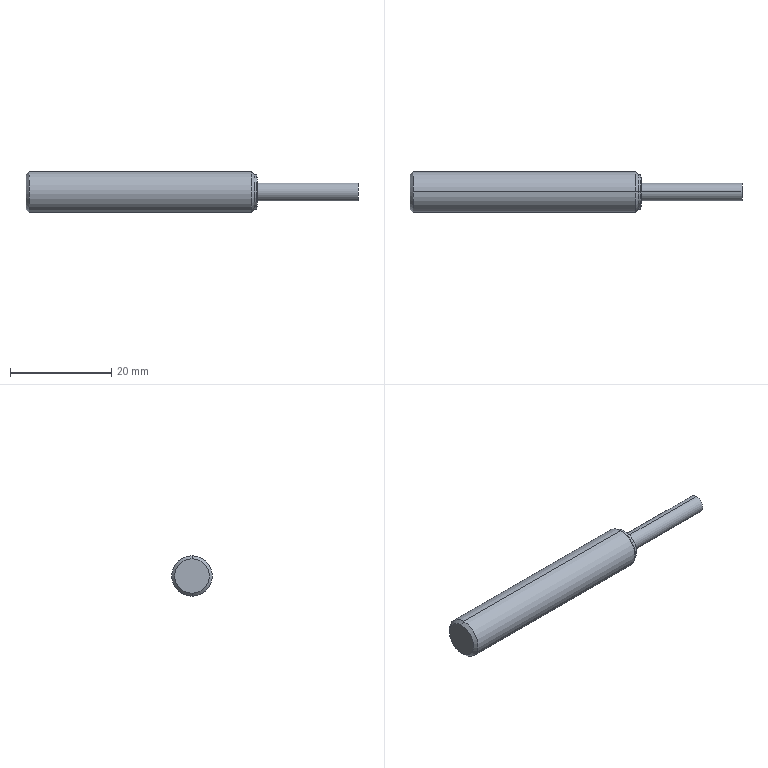Part | STEP file | _PSAM8body_default | 1 solid | 18 faces | box 65.45 x 8 x 8 mm | volume 2463 mm3 | cylinder 8 | cone 4 | plane 4 | spline 2 | commonest cylinder face diameters 3.5 x2 5.714 x2 6.773 x2 8 x2
STEP:
#1=CARTESIAN_POINT('',(0.,0.,0.));
#2=DIRECTION('',(0.,0.,1.));
#3=DIRECTION('',(1.,0.,0.));
#4=AXIS2_PLACEMENT_3D('',#1,#2,#3);
#5=CARTESIAN_POINT('',(45.55,2.286,0.433));
#6=VERTEX_POINT('',#5);
#7=CARTESIAN_POINT('',(45.55,2.286,-0.433));
#8=VERTEX_POINT('',#7);
#9=CARTESIAN_POINT('',(45.55,2.286,0.));
#10=DIRECTION('',(-1.,0.,0.));
#11=DIRECTION('',(0.,0.,1.));
#12=AXIS2_PLACEMENT_3D('',#9,#10,#11);
#13=CIRCLE('',#12,0.433);
#14=CARTESIAN_POINT('',(45.55,2.286,0.433));
#15=CARTESIAN_POINT('',(45.55,3.152,0.433));
#16=CARTESIAN_POINT('',(45.55,3.152,-0.433));
#17=CARTESIAN_POINT('',(45.55,2.286,-0.433));
#18=CARTESIAN_POINT('',(45.648,2.286,0.3084));
#19=CARTESIAN_POINT('',(45.648,2.903,0.3084));
#20=CARTESIAN_POINT('',(45.648,2.903,-0.3084));
#21=CARTESIAN_POINT('',(45.648,2.286,-0.3084));
#22=CARTESIAN_POINT('',(45.7,2.286,0.1586));
#23=CARTESIAN_POINT('',(45.7,2.603,0.1586));
#24=CARTESIAN_POINT('',(45.7,2.603,-0.1586));
#25=CARTESIAN_POINT('',(45.7,2.286,-0.1586));
#26=CARTESIAN_POINT('',(45.7,2.286,0.));
#27=CARTESIAN_POINT('',(45.7,2.286,0.));
#28=CARTESIAN_POINT('',(45.7,2.286,0.));
#29=CARTESIAN_POINT('',(45.7,2.286,0.));
#30=(BOUNDED_SURFACE()B_SPLINE_SURFACE(3,3,((#14,#15,#16,#17),(#18,#19,#20,#21),(#22,#23,#24,#25),(#26,#27,#28,#29)),.UNSPECIFIED.,.F.,.F.,.F.)B_SPLINE_SURFACE_WITH_KNOTS((4,4),(4,4),(0.,1.),(0.,1.),.PIECEWISE_BEZIER_KNOTS.)GEOMETRIC_REPRESENTATION_ITEM()RATIONAL_B_SPLINE_SURFACE(((1.,0.3333,0.3333,1.),(0.9633,0.3211,0.3211,0.9633),(0.9633,0.3211,0.3211,0.9633),(1.,0.3333,0.3333,1.)))REPRESENTATION_ITEM('')SURFACE());
#31=CARTESIAN_POINT('',(0.,0.));
#32=CARTESIAN_POINT('',(0.,0.02375));
#33=CARTESIAN_POINT('',(0.,0.06805));
#34=CARTESIAN_POINT('',(0.,0.1267));
#35=CARTESIAN_POINT('',(0.,0.1794));
#36=CARTESIAN_POINT('',(0.,0.2276));
#37=CARTESIAN_POINT('',(0.,0.2721));
#38=CARTESIAN_POINT('',(0.,0.3139));
#39=CARTESIAN_POINT('',(0.,0.3535));
#40=CARTESIAN_POINT('',(0.,0.3914));
#41=CARTESIAN_POINT('',(0.,0.4282));
#42=CARTESIAN_POINT('',(0.,0.4643));
#43=CARTESIAN_POINT('',(0.,0.5));
#44=CARTESIAN_POINT('',(0.,0.5357));
#45=CARTESIAN_POINT('',(0.,0.5718));
#46=CARTESIAN_POINT('',(0.,0.6086));
#47=CARTESIAN_POINT('',(0.,0.6465));
#48=CARTESIAN_POINT('',(0.,0.6861));
#49=CARTESIAN_POINT('',(0.,0.7279));
#50=CARTESIAN_POINT('',(0.,0.7724));
#51=CARTESIAN_POINT('',(0.,0.8206));
#52=CARTESIAN_POINT('',(0.,0.8733));
#53=CARTESIAN_POINT('',(0.,0.9319));
#54=CARTESIAN_POINT('',(0.,0.9763));
#55=CARTESIAN_POINT('',(0.,1.));
#56=B_SPLINE_CURVE_WITH_KNOTS('',3,(#31,#32,#33,#34,#35,#36,#37,#38,#39,#40,#41,#42,#43,#44,#45,#46,#47,#48,#49,#50,#51,#52,#53,#54,#55),.UNSPECIFIED.,.F.,.F.,(4,1,1,1,1,1,1,1,1,1,1,1,1,1,1,1,1,1,1,1,1,1,4),(0.,0.1428,0.2856,0.4284,0.5712,0.714,0.8568,0.9996,1.142,1.285,1.428,1.571,1.714,1.856,1.999,2.142,2.285,2.428,2.57,2.713,2.856,2.999,3.142),.QUASI_UNIFORM_KNOTS.);
#57=(GEOMETRIC_REPRESENTATION_CONTEXT(2)PARAMETRIC_REPRESENTATION_CONTEXT()REPRESENTATION_CONTEXT('',''));
#58=DEFINITIONAL_REPRESENTATION('',(#56),#57);
#59=PCURVE('',#30,#58);
#60=CARTESIAN_POINT('',(45.55,0.,0.));
#61=DIRECTION('',(1.,0.,0.));
#62=DIRECTION('',(0.,0.,-1.));
#63=AXIS2_PLACEMENT_3D('',#60,#61,#62);
#64=PLANE('',#63);
#65=CARTESIAN_POINT('',(-0.433,2.286));
#66=CARTESIAN_POINT('',(-0.433,3.036));
#67=CARTESIAN_POINT('',(0.2165,2.661));
#68=CARTESIAN_POINT('',(0.866,2.286));
#69=CARTESIAN_POINT('',(0.2165,1.911));
#70=CARTESIAN_POINT('',(-0.433,1.536));
#71=CARTESIAN_POINT('',(-0.433,2.286));
#72=(BOUNDED_CURVE()B_SPLINE_CURVE(2,(#65,#66,#67,#68,#69,#70,#71),.UNSPECIFIED.,.T.,.F.)B_SPLINE_CURVE_WITH_KNOTS((1,2,2,2,2,1),(-2.094,0.,2.094,4.189,6.283,8.378),.UNSPECIFIED.)CURVE()GEOMETRIC_REPRESENTATION_ITEM()RATIONAL_B_SPLINE_CURVE((1.,0.5,1.,0.5,1.,0.5,1.))REPRESENTATION_ITEM(''));
#73=(GEOMETRIC_REPRESENTATION_CONTEXT(2)PARAMETRIC_REPRESENTATION_CONTEXT()REPRESENTATION_CONTEXT('',''));
#74=DEFINITIONAL_REPRESENTATION('',(#72),#73);
#75=PCURVE('',#64,#74);
#76=SURFACE_CURVE('',#13,(#59,#75),.PCURVE_S1.);
#77=EDGE_CURVE('',#6,#8,#76,.T.);
#78=ORIENTED_EDGE('',*,*,#77,.F.);
#79=CARTESIAN_POINT('',(45.7,2.286,0.));
#80=VERTEX_POINT('',#79);
#81=CARTESIAN_POINT('',(45.,2.286,0.));
#82=DIRECTION('',(0.,1.,0.));
#83=DIRECTION('',(-1.,0.,0.));
#84=AXIS2_PLACEMENT_3D('',#81,#82,#83);
#85=CIRCLE('',#84,0.7);
#86=CARTESIAN_POINT('',(0.,0.));
#87=CARTESIAN_POINT('',(0.01544,0.));
#88=CARTESIAN_POINT('',(0.04623,0.));
#89=CARTESIAN_POINT('',(0.09221,0.));
#90=CARTESIAN_POINT('',(0.138,0.));
#91=CARTESIAN_POINT('',(0.1836,0.));
#92=CARTESIAN_POINT('',(0.2291,0.));
#93=CARTESIAN_POINT('',(0.2744,0.));
#94=CARTESIAN_POINT('',(0.3197,0.));
#95=CARTESIAN_POINT('',(0.3648,0.));
#96=CARTESIAN_POINT('',(0.4099,0.));
#97=CARTESIAN_POINT('',(0.455,0.));
#98=CARTESIAN_POINT('',(0.5,0.));
#99=CARTESIAN_POINT('',(0.545,0.));
#100=CARTESIAN_POINT('',(0.5901,0.));
#101=CARTESIAN_POINT('',(0.6352,0.));
#102=CARTESIAN_POINT('',(0.6803,0.));
#103=CARTESIAN_POINT('',(0.7256,0.));
#104=CARTESIAN_POINT('',(0.7709,0.));
#105=CARTESIAN_POINT('',(0.8164,0.));
#106=CARTESIAN_POINT('',(0.862,0.));
#107=CARTESIAN_POINT('',(0.9078,0.));
#108=CARTESIAN_POINT('',(0.9538,0.));
#109=CARTESIAN_POINT('',(0.9846,0.));
#110=CARTESIAN_POINT('',(1.,0.));
#111=B_SPLINE_CURVE_WITH_KNOTS('',3,(#86,#87,#88,#89,#90,#91,#92,#93,#94,#95,#96,#97,#98,#99,#100,#101,#102,#103,#104,#105,#106,#107,#108,#109,#110),.UNSPECIFIED.,.F.,.F.,(4,1,1,1,1,1,1,1,1,1,1,1,1,1,1,1,1,1,1,1,1,1,4),(2.475,2.505,2.535,2.566,2.596,2.626,2.657,2.687,2.717,2.747,2.778,2.808,2.838,2.869,2.899,2.929,2.96,2.99,3.02,3.051,3.081,3.111,3.142),.QUASI_UNIFORM_KNOTS.);
#112=(GEOMETRIC_REPRESENTATION_CONTEXT(2)PARAMETRIC_REPRESENTATION_CONTEXT()REPRESENTATION_CONTEXT('',''));
#113=DEFINITIONAL_REPRESENTATION('',(#111),#112);
#114=PCURVE('',#30,#113);
#115=CARTESIAN_POINT('',(45.55,2.286,-0.433));
#116=CARTESIAN_POINT('',(45.55,1.42,-0.433));
#117=CARTESIAN_POINT('',(45.55,1.42,0.433));
#118=CARTESIAN_POINT('',(45.55,2.286,0.433));
#119=CARTESIAN_POINT('',(45.648,2.286,-0.3084));
#120=CARTESIAN_POINT('',(45.648,1.669,-0.3084));
#121=CARTESIAN_POINT('',(45.648,1.669,0.3084));
#122=CARTESIAN_POINT('',(45.648,2.286,0.3084));
#123=CARTESIAN_POINT('',(45.7,2.286,-0.1586));
#124=CARTESIAN_POINT('',(45.7,1.969,-0.1586));
#125=CARTESIAN_POINT('',(45.7,1.969,0.1586));
#126=CARTESIAN_POINT('',(45.7,2.286,0.1586));
#127=CARTESIAN_POINT('',(45.7,2.286,0.));
#128=CARTESIAN_POINT('',(45.7,2.286,0.));
#129=CARTESIAN_POINT('',(45.7,2.286,0.));
#130=CARTESIAN_POINT('',(45.7,2.286,0.));
#131=(BOUNDED_SURFACE()B_SPLINE_SURFACE(3,3,((#115,#116,#117,#118),(#119,#120,#121,#122),(#123,#124,#125,#126),(#127,#128,#129,#130)),.UNSPECIFIED.,.F.,.F.,.F.)B_SPLINE_SURFACE_WITH_KNOTS((4,4),(4,4),(0.,1.),(0.,1.),.PIECEWISE_BEZIER_KNOTS.)GEOMETRIC_REPRESENTATION_ITEM()RATIONAL_B_SPLINE_SURFACE(((1.,0.3333,0.3333,1.),(0.9633,0.3211,0.3211,0.9633),(0.9633,0.3211,0.3211,0.9633),(1.,0.3333,0.3333,1.)))REPRESENTATION_ITEM('')SURFACE());
#132=CARTESIAN_POINT('',(0.,1.));
#133=CARTESIAN_POINT('',(0.01544,1.));
#134=CARTESIAN_POINT('',(0.04623,1.));
#135=CARTESIAN_POINT('',(0.09221,1.));
#136=CARTESIAN_POINT('',(0.138,1.));
#137=CARTESIAN_POINT('',(0.1836,1.));
#138=CARTESIAN_POINT('',(0.2291,1.));
#139=CARTESIAN_POINT('',(0.2744,1.));
#140=CARTESIAN_POINT('',(0.3197,1.));
#141=CARTESIAN_POINT('',(0.3648,1.));
#142=CARTESIAN_POINT('',(0.4099,1.));
#143=CARTESIAN_POINT('',(0.455,1.));
#144=CARTESIAN_POINT('',(0.5,1.));
#145=CARTESIAN_POINT('',(0.545,1.));
#146=CARTESIAN_POINT('',(0.5901,1.));
#147=CARTESIAN_POINT('',(0.6352,1.));
#148=CARTESIAN_POINT('',(0.6803,1.));
#149=CARTESIAN_POINT('',(0.7256,1.));
#150=CARTESIAN_POINT('',(0.7709,1.));
#151=CARTESIAN_POINT('',(0.8164,1.));
#152=CARTESIAN_POINT('',(0.862,1.));
#153=CARTESIAN_POINT('',(0.9078,1.));
#154=CARTESIAN_POINT('',(0.9538,1.));
#155=CARTESIAN_POINT('',(0.9846,1.));
#156=CARTESIAN_POINT('',(1.,1.));
#157=B_SPLINE_CURVE_WITH_KNOTS('',3,(#132,#133,#134,#135,#136,#137,#138,#139,#140,#141,#142,#143,#144,#145,#146,#147,#148,#149,#150,#151,#152,#153,#154,#155,#156),.UNSPECIFIED.,.F.,.F.,(4,1,1,1,1,1,1,1,1,1,1,1,1,1,1,1,1,1,1,1,1,1,4),(2.475,2.505,2.535,2.566,2.596,2.626,2.657,2.687,2.717,2.747,2.778,2.808,2.838,2.869,2.899,2.929,2.96,2.99,3.02,3.051,3.081,3.111,3.142),.QUASI_UNIFORM_KNOTS.);
#158=(GEOMETRIC_REPRESENTATION_CONTEXT(2)PARAMETRIC_REPRESENTATION_CONTEXT()REPRESENTATION_CONTEXT('',''));
#159=DEFINITIONAL_REPRESENTATION('',(#157),#158);
#160=PCURVE('',#131,#159);
#161=SURFACE_CURVE('',#85,(#114,#160),.PCURVE_S1.);
#162=EDGE_CURVE('',#6,#80,#161,.T.);
#163=ORIENTED_EDGE('',*,*,#162,.T.);
#164=CARTESIAN_POINT('',(45.,2.286,0.));
#165=DIRECTION('',(0.,-1.,0.));
#166=DIRECTION('',(-1.,0.,0.));
#167=AXIS2_PLACEMENT_3D('',#164,#165,#166);
#168=CIRCLE('',#167,0.7);
#169=CARTESIAN_POINT('',(0.,1.));
#170=CARTESIAN_POINT('',(0.01544,1.));
#171=CARTESIAN_POINT('',(0.04623,1.));
#172=CARTESIAN_POINT('',(0.09221,1.));
#173=CARTESIAN_POINT('',(0.138,1.));
#174=CARTESIAN_POINT('',(0.1836,1.));
#175=CARTESIAN_POINT('',(0.2291,1.));
#176=CARTESIAN_POINT('',(0.2744,1.));
#177=CARTESIAN_POINT('',(0.3197,1.));
#178=CARTESIAN_POINT('',(0.3648,1.));
#179=CARTESIAN_POINT('',(0.4099,1.));
#180=CARTESIAN_POINT('',(0.455,1.));
#181=CARTESIAN_POINT('',(0.5,1.));
#182=CARTESIAN_POINT('',(0.545,1.));
#183=CARTESIAN_POINT('',(0.5901,1.));
#184=CARTESIAN_POINT('',(0.6352,1.));
#185=CARTESIAN_POINT('',(0.6803,1.));
#186=CARTESIAN_POINT('',(0.7256,1.));
#187=CARTESIAN_POINT('',(0.7709,1.));
#188=CARTESIAN_POINT('',(0.8164,1.));
#189=CARTESIAN_POINT('',(0.862,1.));
#190=CARTESIAN_POINT('',(0.9078,1.));
#191=CARTESIAN_POINT('',(0.9538,1.));
#192=CARTESIAN_POINT('',(0.9846,1.));
#193=CARTESIAN_POINT('',(1.,1.));
#194=B_SPLINE_CURVE_WITH_KNOTS('',3,(#169,#170,#171,#172,#173,#174,#175,#176,#177,#178,#179,#180,#181,#182,#183,#184,#185,#186,#187,#188,#189,#190,#191,#192,#193),.UNSPECIFIED.,.F.,.F.,(4,1,1,1,1,1,1,1,1,1,1,1,1,1,1,1,1,1,1,1,1,1,4),(2.475,2.505,2.535,2.566,2.596,2.626,2.657,2.687,2.717,2.747,2.778,2.808,2.838,2.869,2.899,2.929,2.96,2.99,3.02,3.051,3.081,3.111,3.142),.QUASI_UNIFORM_KNOTS.);
#195=(GEOMETRIC_REPRESENTATION_CONTEXT(2)PARAMETRIC_REPRESENTATION_CONTEXT()REPRESENTATION_CONTEXT('',''));
#196=DEFINITIONAL_REPRESENTATION('',(#194),#195);
#197=PCURVE('',#30,#196);
#198=CARTESIAN_POINT('',(0.,0.));
#199=CARTESIAN_POINT('',(0.01544,0.));
#200=CARTESIAN_POINT('',(0.04623,0.));
#201=CARTESIAN_POINT('',(0.09221,0.));
#202=CARTESIAN_POINT('',(0.138,0.));
#203=CARTESIAN_POINT('',(0.1836,0.));
#204=CARTESIAN_POINT('',(0.2291,0.));
#205=CARTESIAN_POINT('',(0.2744,0.));
#206=CARTESIAN_POINT('',(0.3197,0.));
#207=CARTESIAN_POINT('',(0.3648,0.));
#208=CARTESIAN_POINT('',(0.4099,0.));
#209=CARTESIAN_POINT('',(0.455,0.));
#210=CARTESIAN_POINT('',(0.5,0.));
#211=CARTESIAN_POINT('',(0.545,0.));
#212=CARTESIAN_POINT('',(0.5901,0.));
#213=CARTESIAN_POINT('',(0.6352,0.));
#214=CARTESIAN_POINT('',(0.6803,0.));
#215=CARTESIAN_POINT('',(0.7256,0.));
#216=CARTESIAN_POINT('',(0.7709,0.));
#217=CARTESIAN_POINT('',(0.8164,0.));
#218=CARTESIAN_POINT('',(0.862,0.));
#219=CARTESIAN_POINT('',(0.9078,0.));
#220=CARTESIAN_POINT('',(0.9538,0.));
#221=CARTESIAN_POINT('',(0.9846,0.));
#222=CARTESIAN_POINT('',(1.,0.));
#223=B_SPLINE_CURVE_WITH_KNOTS('',3,(#198,#199,#200,#201,#202,#203,#204,#205,#206,#207,#208,#209,#210,#211,#212,#213,#214,#215,#216,#217,#218,#219,#220,#221,#222),.UNSPECIFIED.,.F.,.F.,(4,1,1,1,1,1,1,1,1,1,1,1,1,1,1,1,1,1,1,1,1,1,4),(2.475,2.505,2.535,2.566,2.596,2.626,2.657,2.687,2.717,2.747,2.778,2.808,2.838,2.869,2.899,2.929,2.96,2.99,3.02,3.051,3.081,3.111,3.142),.QUASI_UNIFORM_KNOTS.);
#224=(GEOMETRIC_REPRESENTATION_CONTEXT(2)PARAMETRIC_REPRESENTATION_CONTEXT()REPRESENTATION_CONTEXT('',''));
#225=DEFINITIONAL_REPRESENTATION('',(#223),#224);
#226=PCURVE('',#131,#225);
#227=SURFACE_CURVE('',#168,(#197,#226),.PCURVE_S1.);
#228=EDGE_CURVE('',#8,#80,#227,.T.);
#229=ORIENTED_EDGE('',*,*,#228,.F.);
#230=EDGE_LOOP('',(#78,#163,#229));
#231=FACE_BOUND('',#230,.T.);
#232=ADVANCED_FACE('',(#231),#30,.T.);
#233=CARTESIAN_POINT('',(44.386,0.,4.));
#234=VERTEX_POINT('',#233);
#235=CARTESIAN_POINT('',(44.386,0.,-4.));
#236=VERTEX_POINT('',#235);
#237=CARTESIAN_POINT('',(44.386,0.,0.));
#238=DIRECTION('',(-1.,0.,0.));
#239=DIRECTION('',(0.,0.,1.));
#240=AXIS2_PLACEMENT_3D('',#237,#238,#239);
#241=CIRCLE('',#240,4.);
#242=CARTESIAN_POINT('',(65.45,0.,0.));
#243=DIRECTION('',(-1.,0.,0.));
#244=DIRECTION('',(0.,0.,1.));
#245=AXIS2_PLACEMENT_3D('',#242,#243,#244);
#246=CYLINDRICAL_SURFACE('',#245,4.);
#247=CARTESIAN_POINT('',(0.,21.064));
#248=DIRECTION('',(1.,0.));
#249=VECTOR('',#248,1.);
#250=LINE('',#247,#249);
#251=(GEOMETRIC_REPRESENTATION_CONTEXT(2)PARAMETRIC_REPRESENTATION_CONTEXT()REPRESENTATION_CONTEXT('',''));
#252=DEFINITIONAL_REPRESENTATION('',(#250),#251);
#253=PCURVE('',#246,#252);
#254=CARTESIAN_POINT('',(44.387,0.,0.));
#255=DIRECTION('',(-1.,0.,0.));
#256=DIRECTION('',(0.,0.,1.));
#257=AXIS2_PLACEMENT_3D('',#254,#255,#256);
#258=CONICAL_SURFACE('',#257,4.,0.7854);
#259=CARTESIAN_POINT('',(0.,0.));
#260=DIRECTION('',(1.,0.));
#261=VECTOR('',#260,1.);
#262=LINE('',#259,#261);
#263=(GEOMETRIC_REPRESENTATION_CONTEXT(2)PARAMETRIC_REPRESENTATION_CONTEXT()REPRESENTATION_CONTEXT('',''));
#264=DEFINITIONAL_REPRESENTATION('',(#262),#263);
#265=PCURVE('',#258,#264);
#266=SURFACE_CURVE('',#241,(#253,#265),.PCURVE_S1.);
#267=EDGE_CURVE('',#234,#236,#266,.T.);
#268=ORIENTED_EDGE('',*,*,#267,.T.);
#269=CARTESIAN_POINT('',(0.6135,0.,-4.));
#270=VERTEX_POINT('',#269);
#271=CARTESIAN_POINT('',(65.45,0.,-4.));
#272=DIRECTION('',(-1.,0.,0.));
#273=VECTOR('',#272,1.);
#274=LINE('',#271,#273);
#275=CARTESIAN_POINT('',(3.142,0.));
#276=DIRECTION('',(0.,1.));
#277=VECTOR('',#276,1.);
#278=LINE('',#275,#277);
#279=(GEOMETRIC_REPRESENTATION_CONTEXT(2)PARAMETRIC_REPRESENTATION_CONTEXT()REPRESENTATION_CONTEXT('',''));
#280=DEFINITIONAL_REPRESENTATION('',(#278),#279);
#281=PCURVE('',#246,#280);
#282=CARTESIAN_POINT('',(65.45,0.,0.));
#283=DIRECTION('',(-1.,0.,0.));
#284=DIRECTION('',(0.,0.,1.));
#285=AXIS2_PLACEMENT_3D('',#282,#283,#284);
#286=CYLINDRICAL_SURFACE('',#285,4.);
#287=CARTESIAN_POINT('',(3.142,0.));
#288=DIRECTION('',(0.,1.));
#289=VECTOR('',#288,1.);
#290=LINE('',#287,#289);
#291=(GEOMETRIC_REPRESENTATION_CONTEXT(2)PARAMETRIC_REPRESENTATION_CONTEXT()REPRESENTATION_CONTEXT('',''));
#292=DEFINITIONAL_REPRESENTATION('',(#290),#291);
#293=PCURVE('',#286,#292);
#294=SURFACE_CURVE('',#274,(#281,#293),.PCURVE_S1.);
#295=EDGE_CURVE('',#236,#270,#294,.T.);
#296=ORIENTED_EDGE('',*,*,#295,.T.);
#297=CARTESIAN_POINT('',(0.6135,0.,4.));
#298=VERTEX_POINT('',#297);
#299=CARTESIAN_POINT('',(0.6135,0.,0.));
#300=DIRECTION('',(1.,0.,0.));
#301=DIRECTION('',(0.,0.,1.));
#302=AXIS2_PLACEMENT_3D('',#299,#300,#301);
#303=CIRCLE('',#302,4.);
#304=CARTESIAN_POINT('',(6.283,64.837));
#305=DIRECTION('',(-1.,0.));
#306=VECTOR('',#305,1.);
#307=LINE('',#304,#306);
#308=(GEOMETRIC_REPRESENTATION_CONTEXT(2)PARAMETRIC_REPRESENTATION_CONTEXT()REPRESENTATION_CONTEXT('',''));
#309=DEFINITIONAL_REPRESENTATION('',(#307),#308);
#310=PCURVE('',#246,#309);
#311=CARTESIAN_POINT('',(0.6135,0.,0.));
#312=DIRECTION('',(1.,0.,0.));
#313=DIRECTION('',(0.,0.,-1.));
#314=AXIS2_PLACEMENT_3D('',#311,#312,#313);
#315=CONICAL_SURFACE('',#314,4.,0.7854);
#316=CARTESIAN_POINT('',(-3.142,0.));
#317=DIRECTION('',(1.,0.));
#318=VECTOR('',#317,1.);
#319=LINE('',#316,#318);
#320=(GEOMETRIC_REPRESENTATION_CONTEXT(2)PARAMETRIC_REPRESENTATION_CONTEXT()REPRESENTATION_CONTEXT('',''));
#321=DEFINITIONAL_REPRESENTATION('',(#319),#320);
#322=PCURVE('',#315,#321);
#323=SURFACE_CURVE('',#303,(#310,#322),.PCURVE_S1.);
#324=EDGE_CURVE('',#270,#298,#323,.T.);
#325=ORIENTED_EDGE('',*,*,#324,.T.);
#326=CARTESIAN_POINT('',(65.45,0.,4.));
#327=DIRECTION('',(-1.,0.,0.));
#328=VECTOR('',#327,1.);
#329=LINE('',#326,#328);
#330=CARTESIAN_POINT('',(0.,0.));
#331=DIRECTION('',(0.,1.));
#332=VECTOR('',#331,1.);
#333=LINE('',#330,#332);
#334=(GEOMETRIC_REPRESENTATION_CONTEXT(2)PARAMETRIC_REPRESENTATION_CONTEXT()REPRESENTATION_CONTEXT('',''));
#335=DEFINITIONAL_REPRESENTATION('',(#333),#334);
#336=PCURVE('',#246,#335);
#337=CARTESIAN_POINT('',(6.283,0.));
#338=DIRECTION('',(0.,1.));
#339=VECTOR('',#338,1.);
#340=LINE('',#337,#339);
#341=(GEOMETRIC_REPRESENTATION_CONTEXT(2)PARAMETRIC_REPRESENTATION_CONTEXT()REPRESENTATION_CONTEXT('',''));
#342=DEFINITIONAL_REPRESENTATION('',(#340),#341);
#343=PCURVE('',#286,#342);
#344=SURFACE_CURVE('',#329,(#336,#343),.PCURVE_S1.);
#345=EDGE_CURVE('',#234,#298,#344,.T.);
#346=ORIENTED_EDGE('',*,*,#345,.F.);
#347=EDGE_LOOP('',(#268,#296,#325,#346));
#348=FACE_BOUND('',#347,.T.);
#349=ADVANCED_FACE('',(#348),#246,.T.);
#350=CARTESIAN_POINT('',(0.,0.,-3.386));
#351=VERTEX_POINT('',#350);
#352=CARTESIAN_POINT('',(0.,0.,3.386));
#353=VERTEX_POINT('',#352);
#354=CARTESIAN_POINT('',(0.,0.,0.));
#355=DIRECTION('',(1.,0.,0.));
#356=DIRECTION('',(0.,0.,-1.));
#357=AXIS2_PLACEMENT_3D('',#354,#355,#356);
#358=CIRCLE('',#357,3.386);
#359=CARTESIAN_POINT('',(0.,-0.6135));
#360=DIRECTION('',(1.,0.));
#361=VECTOR('',#360,1.);
#362=LINE('',#359,#361);
#363=(GEOMETRIC_REPRESENTATION_CONTEXT(2)PARAMETRIC_REPRESENTATION_CONTEXT()REPRESENTATION_CONTEXT('',''));
#364=DEFINITIONAL_REPRESENTATION('',(#362),#363);
#365=PCURVE('',#315,#364);
#366=CARTESIAN_POINT('',(0.,0.,0.));
#367=DIRECTION('',(1.,0.,0.));
#368=DIRECTION('',(0.,0.,-1.));
#369=AXIS2_PLACEMENT_3D('',#366,#367,#368);
#370=PLANE('',#369);
#371=CARTESIAN_POINT('',(0.,0.));
#372=DIRECTION('',(1.,0.));
#373=AXIS2_PLACEMENT_2D('',#371,#372);
#374=CIRCLE('',#373,3.386);
#375=(GEOMETRIC_REPRESENTATION_CONTEXT(2)PARAMETRIC_REPRESENTATION_CONTEXT()REPRESENTATION_CONTEXT('',''));
#376=DEFINITIONAL_REPRESENTATION('',(#374),#375);
#377=PCURVE('',#370,#376);
#378=SURFACE_CURVE('',#358,(#365,#377),.PCURVE_S1.);
#379=EDGE_CURVE('',#351,#353,#378,.T.);
#380=ORIENTED_EDGE('',*,*,#379,.T.);
#381=CARTESIAN_POINT('',(0.6135,0.,4.));
#382=DIRECTION('',(0.7071,0.,0.7071));
#383=VECTOR('',#382,1.);
#384=LINE('',#381,#383);
#385=CARTESIAN_POINT('',(3.142,0.));
#386=DIRECTION('',(0.,1.));
#387=VECTOR('',#386,1.);
#388=LINE('',#385,#387);
#389=(GEOMETRIC_REPRESENTATION_CONTEXT(2)PARAMETRIC_REPRESENTATION_CONTEXT()REPRESENTATION_CONTEXT('',''));
#390=DEFINITIONAL_REPRESENTATION('',(#388),#389);
#391=PCURVE('',#315,#390);
#392=CARTESIAN_POINT('',(0.6135,0.,0.));
#393=DIRECTION('',(1.,0.,0.));
#394=DIRECTION('',(0.,0.,-1.));
#395=AXIS2_PLACEMENT_3D('',#392,#393,#394);
#396=CONICAL_SURFACE('',#395,4.,0.7854);
#397=CARTESIAN_POINT('',(3.142,0.));
#398=DIRECTION('',(0.,1.));
#399=VECTOR('',#398,1.);
#400=LINE('',#397,#399);
#401=(GEOMETRIC_REPRESENTATION_CONTEXT(2)PARAMETRIC_REPRESENTATION_CONTEXT()REPRESENTATION_CONTEXT('',''));
#402=DEFINITIONAL_REPRESENTATION('',(#400),#401);
#403=PCURVE('',#396,#402);
#404=SURFACE_CURVE('',#384,(#391,#403),.PCURVE_S1.);
#405=EDGE_CURVE('',#353,#298,#404,.T.);
#406=ORIENTED_EDGE('',*,*,#405,.T.);
#407=ORIENTED_EDGE('',*,*,#324,.F.);
#408=CARTESIAN_POINT('',(0.6135,0.,-4.));
#409=DIRECTION('',(0.7071,0.,-0.7071));
#410=VECTOR('',#409,1.);
#411=LINE('',#408,#410);
#412=CARTESIAN_POINT('',(0.,0.));
#413=DIRECTION('',(0.,1.));
#414=VECTOR('',#413,1.);
#415=LINE('',#412,#414);
#416=(GEOMETRIC_REPRESENTATION_CONTEXT(2)PARAMETRIC_REPRESENTATION_CONTEXT()REPRESENTATION_CONTEXT('',''));
#417=DEFINITIONAL_REPRESENTATION('',(#415),#416);
#418=PCURVE('',#315,#417);
#419=CARTESIAN_POINT('',(6.283,0.));
#420=DIRECTION('',(0.,1.));
#421=VECTOR('',#420,1.);
#422=LINE('',#419,#421);
#423=(GEOMETRIC_REPRESENTATION_CONTEXT(2)PARAMETRIC_REPRESENTATION_CONTEXT()REPRESENTATION_CONTEXT('',''));
#424=DEFINITIONAL_REPRESENTATION('',(#422),#423);
#425=PCURVE('',#396,#424);
#426=SURFACE_CURVE('',#411,(#418,#425),.PCURVE_S1.);
#427=EDGE_CURVE('',#351,#270,#426,.T.);
#428=ORIENTED_EDGE('',*,*,#427,.F.);
#429=EDGE_LOOP('',(#380,#406,#407,#428));
#430=FACE_BOUND('',#429,.T.);
#431=ADVANCED_FACE('',(#430),#315,.T.);
#432=CARTESIAN_POINT('',(45.,0.,3.386));
#433=VERTEX_POINT('',#432);
#434=CARTESIAN_POINT('',(45.,0.,-3.386));
#435=VERTEX_POINT('',#434);
#436=CARTESIAN_POINT('',(45.,0.,0.));
#437=DIRECTION('',(-1.,0.,0.));
#438=DIRECTION('',(0.,0.,1.));
#439=AXIS2_PLACEMENT_3D('',#436,#437,#438);
#440=CIRCLE('',#439,3.386);
#441=CARTESIAN_POINT('',(0.,-0.6135));
#442=DIRECTION('',(1.,0.));
#443=VECTOR('',#442,1.);
#444=LINE('',#441,#443);
#445=(GEOMETRIC_REPRESENTATION_CONTEXT(2)PARAMETRIC_REPRESENTATION_CONTEXT()REPRESENTATION_CONTEXT('',''));
#446=DEFINITIONAL_REPRESENTATION('',(#444),#445);
#447=PCURVE('',#258,#446);
#448=CARTESIAN_POINT('',(65.45,0.,0.));
#449=DIRECTION('',(-1.,0.,0.));
#450=DIRECTION('',(0.,0.,1.));
#451=AXIS2_PLACEMENT_3D('',#448,#449,#450);
#452=CYLINDRICAL_SURFACE('',#451,3.386);
#453=CARTESIAN_POINT('',(0.,20.45));
#454=DIRECTION('',(1.,0.));
#455=VECTOR('',#454,1.);
#456=LINE('',#453,#455);
#457=(GEOMETRIC_REPRESENTATION_CONTEXT(2)PARAMETRIC_REPRESENTATION_CONTEXT()REPRESENTATION_CONTEXT('',''));
#458=DEFINITIONAL_REPRESENTATION('',(#456),#457);
#459=PCURVE('',#452,#458);
#460=SURFACE_CURVE('',#440,(#447,#459),.PCURVE_S1.);
#461=EDGE_CURVE('',#433,#435,#460,.T.);
#462=ORIENTED_EDGE('',*,*,#461,.T.);
#463=CARTESIAN_POINT('',(44.387,0.,-4.));
#464=DIRECTION('',(-0.7071,0.,-0.7071));
#465=VECTOR('',#464,1.);
#466=LINE('',#463,#465);
#467=CARTESIAN_POINT('',(3.142,0.));
#468=DIRECTION('',(0.,1.));
#469=VECTOR('',#468,1.);
#470=LINE('',#467,#469);
#471=(GEOMETRIC_REPRESENTATION_CONTEXT(2)PARAMETRIC_REPRESENTATION_CONTEXT()REPRESENTATION_CONTEXT('',''));
#472=DEFINITIONAL_REPRESENTATION('',(#470),#471);
#473=PCURVE('',#258,#472);
#474=CARTESIAN_POINT('',(44.387,0.,0.));
#475=DIRECTION('',(-1.,0.,0.));
#476=DIRECTION('',(0.,0.,1.));
#477=AXIS2_PLACEMENT_3D('',#474,#475,#476);
#478=CONICAL_SURFACE('',#477,4.,0.7854);
#479=CARTESIAN_POINT('',(3.142,0.));
#480=DIRECTION('',(0.,1.));
#481=VECTOR('',#480,1.);
#482=LINE('',#479,#481);
#483=(GEOMETRIC_REPRESENTATION_CONTEXT(2)PARAMETRIC_REPRESENTATION_CONTEXT()REPRESENTATION_CONTEXT('',''));
#484=DEFINITIONAL_REPRESENTATION('',(#482),#483);
#485=PCURVE('',#478,#484);
#486=SURFACE_CURVE('',#466,(#473,#485),.PCURVE_S1.);
#487=EDGE_CURVE('',#435,#236,#486,.T.);
#488=ORIENTED_EDGE('',*,*,#487,.T.);
#489=ORIENTED_EDGE('',*,*,#267,.F.);
#490=CARTESIAN_POINT('',(44.387,0.,4.));
#491=DIRECTION('',(-0.7071,0.,0.7071));
#492=VECTOR('',#491,1.);
#493=LINE('',#490,#492);
#494=CARTESIAN_POINT('',(0.,0.));
#495=DIRECTION('',(0.,1.));
#496=VECTOR('',#495,1.);
#497=LINE('',#494,#496);
#498=(GEOMETRIC_REPRESENTATION_CONTEXT(2)PARAMETRIC_REPRESENTATION_CONTEXT()REPRESENTATION_CONTEXT('',''));
#499=DEFINITIONAL_REPRESENTATION('',(#497),#498);
#500=PCURVE('',#258,#499);
#501=CARTESIAN_POINT('',(6.283,0.));
#502=DIRECTION('',(0.,1.));
#503=VECTOR('',#502,1.);
#504=LINE('',#501,#503);
#505=(GEOMETRIC_REPRESENTATION_CONTEXT(2)PARAMETRIC_REPRESENTATION_CONTEXT()REPRESENTATION_CONTEXT('',''));
#506=DEFINITIONAL_REPRESENTATION('',(#504),#505);
#507=PCURVE('',#478,#506);
#508=SURFACE_CURVE('',#493,(#500,#507),.PCURVE_S1.);
#509=EDGE_CURVE('',#433,#234,#508,.T.);
#510=ORIENTED_EDGE('',*,*,#509,.F.);
#511=EDGE_LOOP('',(#462,#488,#489,#510));
#512=FACE_BOUND('',#511,.T.);
#513=ADVANCED_FACE('',(#512),#258,.T.);
#514=CARTESIAN_POINT('',(45.45,0.,3.386));
#515=VERTEX_POINT('',#514);
#516=CARTESIAN_POINT('',(45.45,0.,-3.386));
#517=VERTEX_POINT('',#516);
#518=CARTESIAN_POINT('',(45.45,0.,0.));
#519=DIRECTION('',(-1.,0.,0.));
#520=DIRECTION('',(0.,0.,1.));
#521=AXIS2_PLACEMENT_3D('',#518,#519,#520);
#522=CIRCLE('',#521,3.386);
#523=CARTESIAN_POINT('',(0.,20.));
#524=DIRECTION('',(1.,0.));
#525=VECTOR('',#524,1.);
#526=LINE('',#523,#525);
#527=(GEOMETRIC_REPRESENTATION_CONTEXT(2)PARAMETRIC_REPRESENTATION_CONTEXT()REPRESENTATION_CONTEXT('',''));
#528=DEFINITIONAL_REPRESENTATION('',(#526),#527);
#529=PCURVE('',#452,#528);
#530=CARTESIAN_POINT('',(45.45,3.386,0.));
#531=DIRECTION('',(-1.,0.,0.));
#532=DIRECTION('',(0.,0.,1.));
#533=AXIS2_PLACEMENT_3D('',#530,#531,#532);
#534=PLANE('',#533);
#535=CARTESIAN_POINT('',(0.,-3.386));
#536=DIRECTION('',(1.,0.));
#537=AXIS2_PLACEMENT_2D('',#535,#536);
#538=CIRCLE('',#537,3.386);
#539=(GEOMETRIC_REPRESENTATION_CONTEXT(2)PARAMETRIC_REPRESENTATION_CONTEXT()REPRESENTATION_CONTEXT('',''));
#540=DEFINITIONAL_REPRESENTATION('',(#538),#539);
#541=PCURVE('',#534,#540);
#542=SURFACE_CURVE('',#522,(#529,#541),.PCURVE_S1.);
#543=EDGE_CURVE('',#515,#517,#542,.T.);
#544=ORIENTED_EDGE('',*,*,#543,.T.);
#545=CARTESIAN_POINT('',(65.45,0.,-3.386));
#546=DIRECTION('',(-1.,0.,0.));
#547=VECTOR('',#546,1.);
#548=LINE('',#545,#547);
#549=CARTESIAN_POINT('',(3.142,0.));
#550=DIRECTION('',(0.,1.));
#551=VECTOR('',#550,1.);
#552=LINE('',#549,#551);
#553=(GEOMETRIC_REPRESENTATION_CONTEXT(2)PARAMETRIC_REPRESENTATION_CONTEXT()REPRESENTATION_CONTEXT('',''));
#554=DEFINITIONAL_REPRESENTATION('',(#552),#553);
#555=PCURVE('',#452,#554);
#556=CARTESIAN_POINT('',(65.45,0.,0.));
#557=DIRECTION('',(-1.,0.,0.));
#558=DIRECTION('',(0.,0.,1.));
#559=AXIS2_PLACEMENT_3D('',#556,#557,#558);
#560=CYLINDRICAL_SURFACE('',#559,3.386);
#561=CARTESIAN_POINT('',(3.142,0.));
#562=DIRECTION('',(0.,1.));
#563=VECTOR('',#562,1.);
#564=LINE('',#561,#563);
#565=(GEOMETRIC_REPRESENTATION_CONTEXT(2)PARAMETRIC_REPRESENTATION_CONTEXT()REPRESENTATION_CONTEXT('',''));
#566=DEFINITIONAL_REPRESENTATION('',(#564),#565);
#567=PCURVE('',#560,#566);
#568=SURFACE_CURVE('',#548,(#555,#567),.PCURVE_S1.);
#569=EDGE_CURVE('',#517,#435,#568,.T.);
#570=ORIENTED_EDGE('',*,*,#569,.T.);
#571=ORIENTED_EDGE('',*,*,#461,.F.);
#572=CARTESIAN_POINT('',(65.45,0.,3.386));
#573=DIRECTION('',(-1.,0.,0.));
#574=VECTOR('',#573,1.);
#575=LINE('',#572,#574);
#576=CARTESIAN_POINT('',(0.,0.));
#577=DIRECTION('',(0.,1.));
#578=VECTOR('',#577,1.);
#579=LINE('',#576,#578);
#580=(GEOMETRIC_REPRESENTATION_CONTEXT(2)PARAMETRIC_REPRESENTATION_CONTEXT()REPRESENTATION_CONTEXT('',''));
#581=DEFINITIONAL_REPRESENTATION('',(#579),#580);
#582=PCURVE('',#452,#581);
#583=CARTESIAN_POINT('',(6.283,0.));
#584=DIRECTION('',(0.,1.));
#585=VECTOR('',#584,1.);
#586=LINE('',#583,#585);
#587=(GEOMETRIC_REPRESENTATION_CONTEXT(2)PARAMETRIC_REPRESENTATION_CONTEXT()REPRESENTATION_CONTEXT('',''));
#588=DEFINITIONAL_REPRESENTATION('',(#586),#587);
#589=PCURVE('',#560,#588);
#590=SURFACE_CURVE('',#575,(#582,#589),.PCURVE_S1.);
#591=EDGE_CURVE('',#515,#433,#590,.T.);
#592=ORIENTED_EDGE('',*,*,#591,.F.);
#593=EDGE_LOOP('',(#544,#570,#571,#592));
#594=FACE_BOUND('',#593,.T.);
#595=ADVANCED_FACE('',(#594),#452,.T.);
#596=CARTESIAN_POINT('',(45.45,0.,-2.857));
#597=VERTEX_POINT('',#596);
#598=CARTESIAN_POINT('',(45.45,0.,2.857));
#599=VERTEX_POINT('',#598);
#600=CARTESIAN_POINT('',(45.45,0.,0.));
#601=DIRECTION('',(1.,0.,0.));
#602=DIRECTION('',(0.,0.,-1.));
#603=AXIS2_PLACEMENT_3D('',#600,#601,#602);
#604=CIRCLE('',#603,2.857);
#605=CARTESIAN_POINT('',(45.55,0.,0.));
#606=DIRECTION('',(1.,0.,0.));
#607=DIRECTION('',(0.,0.,-1.));
#608=AXIS2_PLACEMENT_3D('',#605,#606,#607);
#609=CYLINDRICAL_SURFACE('',#608,2.857);
#610=CARTESIAN_POINT('',(0.,-0.1));
#611=DIRECTION('',(1.,0.));
#612=VECTOR('',#611,1.);
#613=LINE('',#610,#612);
#614=(GEOMETRIC_REPRESENTATION_CONTEXT(2)PARAMETRIC_REPRESENTATION_CONTEXT()REPRESENTATION_CONTEXT('',''));
#615=DEFINITIONAL_REPRESENTATION('',(#613),#614);
#616=PCURVE('',#609,#615);
#617=CARTESIAN_POINT('',(-2.857,-3.386));
#618=CARTESIAN_POINT('',(-2.857,1.562));
#619=CARTESIAN_POINT('',(1.429,-0.9121));
#620=CARTESIAN_POINT('',(5.714,-3.386));
#621=CARTESIAN_POINT('',(1.429,-5.861));
#622=CARTESIAN_POINT('',(-2.857,-8.335));
#623=CARTESIAN_POINT('',(-2.857,-3.386));
#624=(BOUNDED_CURVE()B_SPLINE_CURVE(2,(#617,#618,#619,#620,#621,#622,#623),.UNSPECIFIED.,.T.,.F.)B_SPLINE_CURVE_WITH_KNOTS((1,2,2,2,2,1),(-2.094,0.,2.094,4.189,6.283,8.378),.UNSPECIFIED.)CURVE()GEOMETRIC_REPRESENTATION_ITEM()RATIONAL_B_SPLINE_CURVE((1.,0.5,1.,0.5,1.,0.5,1.))REPRESENTATION_ITEM(''));
#625=(GEOMETRIC_REPRESENTATION_CONTEXT(2)PARAMETRIC_REPRESENTATION_CONTEXT()REPRESENTATION_CONTEXT('',''));
#626=DEFINITIONAL_REPRESENTATION('',(#624),#625);
#627=PCURVE('',#534,#626);
#628=SURFACE_CURVE('',#604,(#616,#627),.PCURVE_S1.);
#629=EDGE_CURVE('',#597,#599,#628,.T.);
#630=ORIENTED_EDGE('',*,*,#629,.T.);
#631=CARTESIAN_POINT('',(45.55,0.,2.857));
#632=VERTEX_POINT('',#631);
#633=CARTESIAN_POINT('',(45.55,0.,2.857));
#634=DIRECTION('',(1.,0.,0.));
#635=VECTOR('',#634,1.);
#636=LINE('',#633,#635);
#637=CARTESIAN_POINT('',(3.142,0.));
#638=DIRECTION('',(0.,1.));
#639=VECTOR('',#638,1.);
#640=LINE('',#637,#639);
#641=(GEOMETRIC_REPRESENTATION_CONTEXT(2)PARAMETRIC_REPRESENTATION_CONTEXT()REPRESENTATION_CONTEXT('',''));
#642=DEFINITIONAL_REPRESENTATION('',(#640),#641);
#643=PCURVE('',#609,#642);
#644=CARTESIAN_POINT('',(45.55,0.,0.));
#645=DIRECTION('',(1.,0.,0.));
#646=DIRECTION('',(0.,0.,-1.));
#647=AXIS2_PLACEMENT_3D('',#644,#645,#646);
#648=CYLINDRICAL_SURFACE('',#647,2.857);
#649=CARTESIAN_POINT('',(3.142,0.));
#650=DIRECTION('',(0.,1.));
#651=VECTOR('',#650,1.);
#652=LINE('',#649,#651);
#653=(GEOMETRIC_REPRESENTATION_CONTEXT(2)PARAMETRIC_REPRESENTATION_CONTEXT()REPRESENTATION_CONTEXT('',''));
#654=DEFINITIONAL_REPRESENTATION('',(#652),#653);
#655=PCURVE('',#648,#654);
#656=SURFACE_CURVE('',#636,(#643,#655),.PCURVE_S1.);
#657=EDGE_CURVE('',#599,#632,#656,.T.);
#658=ORIENTED_EDGE('',*,*,#657,.T.);
#659=CARTESIAN_POINT('',(45.55,0.,-2.857));
#660=VERTEX_POINT('',#659);
#661=CARTESIAN_POINT('',(45.55,0.,0.));
#662=DIRECTION('',(-1.,0.,0.));
#663=DIRECTION('',(0.,0.,-1.));
#664=AXIS2_PLACEMENT_3D('',#661,#662,#663);
#665=CIRCLE('',#664,2.857);
#666=CARTESIAN_POINT('',(6.283,0.));
#667=DIRECTION('',(-1.,0.));
#668=VECTOR('',#667,1.);
#669=LINE('',#666,#668);
#670=(GEOMETRIC_REPRESENTATION_CONTEXT(2)PARAMETRIC_REPRESENTATION_CONTEXT()REPRESENTATION_CONTEXT('',''));
#671=DEFINITIONAL_REPRESENTATION('',(#669),#670);
#672=PCURVE('',#609,#671);
#673=CARTESIAN_POINT('',(2.857,0.));
#674=CARTESIAN_POINT('',(2.857,-4.949));
#675=CARTESIAN_POINT('',(-1.429,-2.474));
#676=CARTESIAN_POINT('',(-5.714,0.));
#677=CARTESIAN_POINT('',(-1.429,2.474));
#678=CARTESIAN_POINT('',(2.857,4.949));
#679=CARTESIAN_POINT('',(2.857,0.));
#680=(BOUNDED_CURVE()B_SPLINE_CURVE(2,(#673,#674,#675,#676,#677,#678,#679),.UNSPECIFIED.,.T.,.F.)B_SPLINE_CURVE_WITH_KNOTS((1,2,2,2,2,1),(-2.094,0.,2.094,4.189,6.283,8.378),.UNSPECIFIED.)CURVE()GEOMETRIC_REPRESENTATION_ITEM()RATIONAL_B_SPLINE_CURVE((1.,0.5,1.,0.5,1.,0.5,1.))REPRESENTATION_ITEM(''));
#681=(GEOMETRIC_REPRESENTATION_CONTEXT(2)PARAMETRIC_REPRESENTATION_CONTEXT()REPRESENTATION_CONTEXT('',''));
#682=DEFINITIONAL_REPRESENTATION('',(#680),#681);
#683=PCURVE('',#64,#682);
#684=SURFACE_CURVE('',#665,(#672,#683),.PCURVE_S1.);
#685=EDGE_CURVE('',#632,#660,#684,.T.);
#686=ORIENTED_EDGE('',*,*,#685,.T.);
#687=CARTESIAN_POINT('',(45.55,0.,-2.857));
#688=DIRECTION('',(1.,0.,0.));
#689=VECTOR('',#688,1.);
#690=LINE('',#687,#689);
#691=CARTESIAN_POINT('',(0.,0.));
#692=DIRECTION('',(0.,1.));
#693=VECTOR('',#692,1.);
#694=LINE('',#691,#693);
#695=(GEOMETRIC_REPRESENTATION_CONTEXT(2)PARAMETRIC_REPRESENTATION_CONTEXT()REPRESENTATION_CONTEXT('',''));
#696=DEFINITIONAL_REPRESENTATION('',(#694),#695);
#697=PCURVE('',#609,#696);
#698=CARTESIAN_POINT('',(6.283,0.));
#699=DIRECTION('',(0.,1.));
#700=VECTOR('',#699,1.);
#701=LINE('',#698,#700);
#702=(GEOMETRIC_REPRESENTATION_CONTEXT(2)PARAMETRIC_REPRESENTATION_CONTEXT()REPRESENTATION_CONTEXT('',''));
#703=DEFINITIONAL_REPRESENTATION('',(#701),#702);
#704=PCURVE('',#648,#703);
#705=SURFACE_CURVE('',#690,(#697,#704),.PCURVE_S1.);
#706=EDGE_CURVE('',#597,#660,#705,.T.);
#707=ORIENTED_EDGE('',*,*,#706,.F.);
#708=EDGE_LOOP('',(#630,#658,#686,#707));
#709=FACE_BOUND('',#708,.T.);
#710=ADVANCED_FACE('',(#709),#609,.T.);
#711=CARTESIAN_POINT('',(65.45,0.,1.75));
#712=VERTEX_POINT('',#711);
#713=CARTESIAN_POINT('',(65.45,0.,-1.75));
#714=VERTEX_POINT('',#713);
#715=CARTESIAN_POINT('',(65.45,0.,0.));
#716=DIRECTION('',(-1.,0.,0.));
#717=DIRECTION('',(0.,0.,1.));
#718=AXIS2_PLACEMENT_3D('',#715,#716,#717);
#719=CIRCLE('',#718,1.75);
#720=CARTESIAN_POINT('',(65.45,0.,0.));
#721=DIRECTION('',(-1.,0.,0.));
#722=DIRECTION('',(0.,0.,1.));
#723=AXIS2_PLACEMENT_3D('',#720,#721,#722);
#724=CYLINDRICAL_SURFACE('',#723,1.75);
#725=CARTESIAN_POINT('',(0.,0.));
#726=DIRECTION('',(1.,0.));
#727=VECTOR('',#726,1.);
#728=LINE('',#725,#727);
#729=(GEOMETRIC_REPRESENTATION_CONTEXT(2)PARAMETRIC_REPRESENTATION_CONTEXT()REPRESENTATION_CONTEXT('',''));
#730=DEFINITIONAL_REPRESENTATION('',(#728),#729);
#731=PCURVE('',#724,#730);
#732=CARTESIAN_POINT('',(65.45,1.75,0.));
#733=DIRECTION('',(-1.,0.,0.));
#734=DIRECTION('',(0.,0.,1.));
#735=AXIS2_PLACEMENT_3D('',#732,#733,#734);
#736=PLANE('',#735);
#737=CARTESIAN_POINT('',(0.,-1.75));
#738=DIRECTION('',(1.,0.));
#739=AXIS2_PLACEMENT_2D('',#737,#738);
#740=CIRCLE('',#739,1.75);
#741=(GEOMETRIC_REPRESENTATION_CONTEXT(2)PARAMETRIC_REPRESENTATION_CONTEXT()REPRESENTATION_CONTEXT('',''));
#742=DEFINITIONAL_REPRESENTATION('',(#740),#741);
#743=PCURVE('',#736,#742);
#744=SURFACE_CURVE('',#719,(#731,#743),.PCURVE_S1.);
#745=EDGE_CURVE('',#712,#714,#744,.T.);
#746=ORIENTED_EDGE('',*,*,#745,.T.);
#747=CARTESIAN_POINT('',(45.55,0.,-1.75));
#748=VERTEX_POINT('',#747);
#749=CARTESIAN_POINT('',(65.45,0.,-1.75));
#750=DIRECTION('',(-1.,0.,0.));
#751=VECTOR('',#750,1.);
#752=LINE('',#749,#751);
#753=CARTESIAN_POINT('',(3.142,0.));
#754=DIRECTION('',(0.,1.));
#755=VECTOR('',#754,1.);
#756=LINE('',#753,#755);
#757=(GEOMETRIC_REPRESENTATION_CONTEXT(2)PARAMETRIC_REPRESENTATION_CONTEXT()REPRESENTATION_CONTEXT('',''));
#758=DEFINITIONAL_REPRESENTATION('',(#756),#757);
#759=PCURVE('',#724,#758);
#760=CARTESIAN_POINT('',(65.45,0.,0.));
#761=DIRECTION('',(-1.,0.,0.));
#762=DIRECTION('',(0.,0.,1.));
#763=AXIS2_PLACEMENT_3D('',#760,#761,#762);
#764=CYLINDRICAL_SURFACE('',#763,1.75);
#765=CARTESIAN_POINT('',(3.142,0.));
#766=DIRECTION('',(0.,1.));
#767=VECTOR('',#766,1.);
#768=LINE('',#765,#767);
#769=(GEOMETRIC_REPRESENTATION_CONTEXT(2)PARAMETRIC_REPRESENTATION_CONTEXT()REPRESENTATION_CONTEXT('',''));
#770=DEFINITIONAL_REPRESENTATION('',(#768),#769);
#771=PCURVE('',#764,#770);
#772=SURFACE_CURVE('',#752,(#759,#771),.PCURVE_S1.);
#773=EDGE_CURVE('',#714,#748,#772,.T.);
#774=ORIENTED_EDGE('',*,*,#773,.T.);
#775=CARTESIAN_POINT('',(45.55,0.,1.75));
#776=VERTEX_POINT('',#775);
#777=CARTESIAN_POINT('',(45.55,0.,0.));
#778=DIRECTION('',(-1.,0.,0.));
#779=DIRECTION('',(0.,0.,1.));
#780=AXIS2_PLACEMENT_3D('',#777,#778,#779);
#781=CIRCLE('',#780,1.75);
#782=CARTESIAN_POINT('',(0.,19.9));
#783=DIRECTION('',(1.,0.));
#784=VECTOR('',#783,1.);
#785=LINE('',#782,#784);
#786=(GEOMETRIC_REPRESENTATION_CONTEXT(2)PARAMETRIC_REPRESENTATION_CONTEXT()REPRESENTATION_CONTEXT('',''));
#787=DEFINITIONAL_REPRESENTATION('',(#785),#786);
#788=PCURVE('',#724,#787);
#789=CARTESIAN_POINT('',(-1.75,0.));
#790=CARTESIAN_POINT('',(-1.75,3.031));
#791=CARTESIAN_POINT('',(0.875,1.516));
#792=CARTESIAN_POINT('',(3.5,0.));
#793=CARTESIAN_POINT('',(0.875,-1.516));
#794=CARTESIAN_POINT('',(-1.75,-3.031));
#795=CARTESIAN_POINT('',(-1.75,0.));
#796=(BOUNDED_CURVE()B_SPLINE_CURVE(2,(#789,#790,#791,#792,#793,#794,#795),.UNSPECIFIED.,.T.,.F.)B_SPLINE_CURVE_WITH_KNOTS((1,2,2,2,2,1),(-2.094,0.,2.094,4.189,6.283,8.378),.UNSPECIFIED.)CURVE()GEOMETRIC_REPRESENTATION_ITEM()RATIONAL_B_SPLINE_CURVE((1.,0.5,1.,0.5,1.,0.5,1.))REPRESENTATION_ITEM(''));
#797=(GEOMETRIC_REPRESENTATION_CONTEXT(2)PARAMETRIC_REPRESENTATION_CONTEXT()REPRESENTATION_CONTEXT('',''));
#798=DEFINITIONAL_REPRESENTATION('',(#796),#797);
#799=PCURVE('',#64,#798);
#800=SURFACE_CURVE('',#781,(#788,#799),.PCURVE_S1.);
#801=EDGE_CURVE('',#776,#748,#800,.T.);
#802=ORIENTED_EDGE('',*,*,#801,.F.);
#803=CARTESIAN_POINT('',(65.45,0.,1.75));
#804=DIRECTION('',(-1.,0.,0.));
#805=VECTOR('',#804,1.);
#806=LINE('',#803,#805);
#807=CARTESIAN_POINT('',(0.,0.));
#808=DIRECTION('',(0.,1.));
#809=VECTOR('',#808,1.);
#810=LINE('',#807,#809);
#811=(GEOMETRIC_REPRESENTATION_CONTEXT(2)PARAMETRIC_REPRESENTATION_CONTEXT()REPRESENTATION_CONTEXT('',''));
#812=DEFINITIONAL_REPRESENTATION('',(#810),#811);
#813=PCURVE('',#724,#812);
#814=CARTESIAN_POINT('',(6.283,0.));
#815=DIRECTION('',(0.,1.));
#816=VECTOR('',#815,1.);
#817=LINE('',#814,#816);
#818=(GEOMETRIC_REPRESENTATION_CONTEXT(2)PARAMETRIC_REPRESENTATION_CONTEXT()REPRESENTATION_CONTEXT('',''));
#819=DEFINITIONAL_REPRESENTATION('',(#817),#818);
#820=PCURVE('',#764,#819);
#821=SURFACE_CURVE('',#806,(#813,#820),.PCURVE_S1.);
#822=EDGE_CURVE('',#712,#776,#821,.T.);
#823=ORIENTED_EDGE('',*,*,#822,.F.);
#824=EDGE_LOOP('',(#746,#774,#802,#823));
#825=FACE_BOUND('',#824,.T.);
#826=ADVANCED_FACE('',(#825),#724,.T.);
#827=ORIENTED_EDGE('',*,*,#295,.F.);
#828=CARTESIAN_POINT('',(44.386,0.,0.));
#829=DIRECTION('',(-1.,0.,0.));
#830=DIRECTION('',(0.,0.,1.));
#831=AXIS2_PLACEMENT_3D('',#828,#829,#830);
#832=CIRCLE('',#831,4.);
#833=CARTESIAN_POINT('',(0.,21.064));
#834=DIRECTION('',(1.,0.));
#835=VECTOR('',#834,1.);
#836=LINE('',#833,#835);
#837=(GEOMETRIC_REPRESENTATION_CONTEXT(2)PARAMETRIC_REPRESENTATION_CONTEXT()REPRESENTATION_CONTEXT('',''));
#838=DEFINITIONAL_REPRESENTATION('',(#836),#837);
#839=PCURVE('',#286,#838);
#840=CARTESIAN_POINT('',(0.,0.));
#841=DIRECTION('',(1.,0.));
#842=VECTOR('',#841,1.);
#843=LINE('',#840,#842);
#844=(GEOMETRIC_REPRESENTATION_CONTEXT(2)PARAMETRIC_REPRESENTATION_CONTEXT()REPRESENTATION_CONTEXT('',''));
#845=DEFINITIONAL_REPRESENTATION('',(#843),#844);
#846=PCURVE('',#478,#845);
#847=SURFACE_CURVE('',#832,(#839,#846),.PCURVE_S1.);
#848=EDGE_CURVE('',#236,#234,#847,.T.);
#849=ORIENTED_EDGE('',*,*,#848,.T.);
#850=ORIENTED_EDGE('',*,*,#345,.T.);
#851=CARTESIAN_POINT('',(0.6135,0.,0.));
#852=DIRECTION('',(1.,0.,0.));
#853=DIRECTION('',(0.,0.,1.));
#854=AXIS2_PLACEMENT_3D('',#851,#852,#853);
#855=CIRCLE('',#854,4.);
#856=CARTESIAN_POINT('',(6.283,64.837));
#857=DIRECTION('',(-1.,0.));
#858=VECTOR('',#857,1.);
#859=LINE('',#856,#858);
#860=(GEOMETRIC_REPRESENTATION_CONTEXT(2)PARAMETRIC_REPRESENTATION_CONTEXT()REPRESENTATION_CONTEXT('',''));
#861=DEFINITIONAL_REPRESENTATION('',(#859),#860);
#862=PCURVE('',#286,#861);
#863=CARTESIAN_POINT('',(3.142,0.));
#864=DIRECTION('',(1.,0.));
#865=VECTOR('',#864,1.);
#866=LINE('',#863,#865);
#867=(GEOMETRIC_REPRESENTATION_CONTEXT(2)PARAMETRIC_REPRESENTATION_CONTEXT()REPRESENTATION_CONTEXT('',''));
#868=DEFINITIONAL_REPRESENTATION('',(#866),#867);
#869=PCURVE('',#396,#868);
#870=SURFACE_CURVE('',#855,(#862,#869),.PCURVE_S1.);
#871=EDGE_CURVE('',#298,#270,#870,.T.);
#872=ORIENTED_EDGE('',*,*,#871,.T.);
#873=EDGE_LOOP('',(#827,#849,#850,#872));
#874=FACE_BOUND('',#873,.T.);
#875=ADVANCED_FACE('',(#874),#286,.T.);
#876=ORIENTED_EDGE('',*,*,#405,.F.);
#877=CARTESIAN_POINT('',(0.,0.,0.));
#878=DIRECTION('',(1.,0.,0.));
#879=DIRECTION('',(0.,0.,-1.));
#880=AXIS2_PLACEMENT_3D('',#877,#878,#879);
#881=CIRCLE('',#880,3.386);
#882=CARTESIAN_POINT('',(0.,-0.6135));
#883=DIRECTION('',(1.,0.));
#884=VECTOR('',#883,1.);
#885=LINE('',#882,#884);
#886=(GEOMETRIC_REPRESENTATION_CONTEXT(2)PARAMETRIC_REPRESENTATION_CONTEXT()REPRESENTATION_CONTEXT('',''));
#887=DEFINITIONAL_REPRESENTATION('',(#885),#886);
#888=PCURVE('',#396,#887);
#889=CARTESIAN_POINT('',(0.,0.));
#890=DIRECTION('',(1.,0.));
#891=AXIS2_PLACEMENT_2D('',#889,#890);
#892=CIRCLE('',#891,3.386);
#893=(GEOMETRIC_REPRESENTATION_CONTEXT(2)PARAMETRIC_REPRESENTATION_CONTEXT()REPRESENTATION_CONTEXT('',''));
#894=DEFINITIONAL_REPRESENTATION('',(#892),#893);
#895=PCURVE('',#370,#894);
#896=SURFACE_CURVE('',#881,(#888,#895),.PCURVE_S1.);
#897=EDGE_CURVE('',#353,#351,#896,.T.);
#898=ORIENTED_EDGE('',*,*,#897,.T.);
#899=ORIENTED_EDGE('',*,*,#427,.T.);
#900=ORIENTED_EDGE('',*,*,#871,.F.);
#901=EDGE_LOOP('',(#876,#898,#899,#900));
#902=FACE_BOUND('',#901,.T.);
#903=ADVANCED_FACE('',(#902),#396,.T.);
#904=ORIENTED_EDGE('',*,*,#487,.F.);
#905=CARTESIAN_POINT('',(45.,0.,0.));
#906=DIRECTION('',(-1.,0.,0.));
#907=DIRECTION('',(0.,0.,1.));
#908=AXIS2_PLACEMENT_3D('',#905,#906,#907);
#909=CIRCLE('',#908,3.386);
#910=CARTESIAN_POINT('',(0.,-0.6135));
#911=DIRECTION('',(1.,0.));
#912=VECTOR('',#911,1.);
#913=LINE('',#910,#912);
#914=(GEOMETRIC_REPRESENTATION_CONTEXT(2)PARAMETRIC_REPRESENTATION_CONTEXT()REPRESENTATION_CONTEXT('',''));
#915=DEFINITIONAL_REPRESENTATION('',(#913),#914);
#916=PCURVE('',#478,#915);
#917=CARTESIAN_POINT('',(0.,20.45));
#918=DIRECTION('',(1.,0.));
#919=VECTOR('',#918,1.);
#920=LINE('',#917,#919);
#921=(GEOMETRIC_REPRESENTATION_CONTEXT(2)PARAMETRIC_REPRESENTATION_CONTEXT()REPRESENTATION_CONTEXT('',''));
#922=DEFINITIONAL_REPRESENTATION('',(#920),#921);
#923=PCURVE('',#560,#922);
#924=SURFACE_CURVE('',#909,(#916,#923),.PCURVE_S1.);
#925=EDGE_CURVE('',#435,#433,#924,.T.);
#926=ORIENTED_EDGE('',*,*,#925,.T.);
#927=ORIENTED_EDGE('',*,*,#509,.T.);
#928=ORIENTED_EDGE('',*,*,#848,.F.);
#929=EDGE_LOOP('',(#904,#926,#927,#928));
#930=FACE_BOUND('',#929,.T.);
#931=ADVANCED_FACE('',(#930),#478,.T.);
#932=ORIENTED_EDGE('',*,*,#379,.F.);
#933=ORIENTED_EDGE('',*,*,#897,.F.);
#934=EDGE_LOOP('',(#932,#933));
#935=FACE_BOUND('',#934,.T.);
#936=ADVANCED_FACE('',(#935),#370,.F.);
#937=ORIENTED_EDGE('',*,*,#569,.F.);
#938=CARTESIAN_POINT('',(45.45,0.,0.));
#939=DIRECTION('',(-1.,0.,0.));
#940=DIRECTION('',(0.,0.,1.));
#941=AXIS2_PLACEMENT_3D('',#938,#939,#940);
#942=CIRCLE('',#941,3.386);
#943=CARTESIAN_POINT('',(0.,20.));
#944=DIRECTION('',(1.,0.));
#945=VECTOR('',#944,1.);
#946=LINE('',#943,#945);
#947=(GEOMETRIC_REPRESENTATION_CONTEXT(2)PARAMETRIC_REPRESENTATION_CONTEXT()REPRESENTATION_CONTEXT('',''));
#948=DEFINITIONAL_REPRESENTATION('',(#946),#947);
#949=PCURVE('',#560,#948);
#950=CARTESIAN_POINT('',(0.,-3.386));
#951=DIRECTION('',(1.,0.));
#952=AXIS2_PLACEMENT_2D('',#950,#951);
#953=CIRCLE('',#952,3.386);
#954=(GEOMETRIC_REPRESENTATION_CONTEXT(2)PARAMETRIC_REPRESENTATION_CONTEXT()REPRESENTATION_CONTEXT('',''));
#955=DEFINITIONAL_REPRESENTATION('',(#953),#954);
#956=PCURVE('',#534,#955);
#957=SURFACE_CURVE('',#942,(#949,#956),.PCURVE_S1.);
#958=EDGE_CURVE('',#517,#515,#957,.T.);
#959=ORIENTED_EDGE('',*,*,#958,.T.);
#960=ORIENTED_EDGE('',*,*,#591,.T.);
#961=ORIENTED_EDGE('',*,*,#925,.F.);
#962=EDGE_LOOP('',(#937,#959,#960,#961));
#963=FACE_BOUND('',#962,.T.);
#964=ADVANCED_FACE('',(#963),#560,.T.);
#965=ORIENTED_EDGE('',*,*,#543,.F.);
#966=ORIENTED_EDGE('',*,*,#958,.F.);
#967=EDGE_LOOP('',(#965,#966));
#968=FACE_BOUND('',#967,.T.);
#969=ORIENTED_EDGE('',*,*,#629,.F.);
#970=CARTESIAN_POINT('',(45.45,0.,0.));
#971=DIRECTION('',(1.,0.,0.));
#972=DIRECTION('',(0.,0.,-1.));
#973=AXIS2_PLACEMENT_3D('',#970,#971,#972);
#974=CIRCLE('',#973,2.857);
#975=CARTESIAN_POINT('',(-2.857,-3.386));
#976=CARTESIAN_POINT('',(-2.857,1.562));
#977=CARTESIAN_POINT('',(1.429,-0.9121));
#978=CARTESIAN_POINT('',(5.714,-3.386));
#979=CARTESIAN_POINT('',(1.429,-5.861));
#980=CARTESIAN_POINT('',(-2.857,-8.335));
#981=CARTESIAN_POINT('',(-2.857,-3.386));
#982=(BOUNDED_CURVE()B_SPLINE_CURVE(2,(#975,#976,#977,#978,#979,#980,#981),.UNSPECIFIED.,.T.,.F.)B_SPLINE_CURVE_WITH_KNOTS((1,2,2,2,2,1),(-2.094,0.,2.094,4.189,6.283,8.378),.UNSPECIFIED.)CURVE()GEOMETRIC_REPRESENTATION_ITEM()RATIONAL_B_SPLINE_CURVE((1.,0.5,1.,0.5,1.,0.5,1.))REPRESENTATION_ITEM(''));
#983=(GEOMETRIC_REPRESENTATION_CONTEXT(2)PARAMETRIC_REPRESENTATION_CONTEXT()REPRESENTATION_CONTEXT('',''));
#984=DEFINITIONAL_REPRESENTATION('',(#982),#983);
#985=PCURVE('',#534,#984);
#986=CARTESIAN_POINT('',(0.,-0.1));
#987=DIRECTION('',(1.,0.));
#988=VECTOR('',#987,1.);
#989=LINE('',#986,#988);
#990=(GEOMETRIC_REPRESENTATION_CONTEXT(2)PARAMETRIC_REPRESENTATION_CONTEXT()REPRESENTATION_CONTEXT('',''));
#991=DEFINITIONAL_REPRESENTATION('',(#989),#990);
#992=PCURVE('',#648,#991);
#993=SURFACE_CURVE('',#974,(#985,#992),.PCURVE_S1.);
#994=EDGE_CURVE('',#599,#597,#993,.T.);
#995=ORIENTED_EDGE('',*,*,#994,.F.);
#996=EDGE_LOOP('',(#969,#995));
#997=FACE_BOUND('',#996,.T.);
#998=ADVANCED_FACE('',(#968,#997),#534,.F.);
#999=ORIENTED_EDGE('',*,*,#657,.F.);
#1000=ORIENTED_EDGE('',*,*,#994,.T.);
#1001=ORIENTED_EDGE('',*,*,#706,.T.);
#1002=CARTESIAN_POINT('',(45.55,0.,0.));
#1003=DIRECTION('',(-1.,0.,0.));
#1004=DIRECTION('',(0.,0.,-1.));
#1005=AXIS2_PLACEMENT_3D('',#1002,#1003,#1004);
#1006=CIRCLE('',#1005,2.857);
#1007=CARTESIAN_POINT('',(6.283,0.));
#1008=DIRECTION('',(-1.,0.));
#1009=VECTOR('',#1008,1.);
#1010=LINE('',#1007,#1009);
#1011=(GEOMETRIC_REPRESENTATION_CONTEXT(2)PARAMETRIC_REPRESENTATION_CONTEXT()REPRESENTATION_CONTEXT('',''));
#1012=DEFINITIONAL_REPRESENTATION('',(#1010),#1011);
#1013=PCURVE('',#648,#1012);
#1014=CARTESIAN_POINT('',(2.857,0.));
#1015=CARTESIAN_POINT('',(2.857,-4.949));
#1016=CARTESIAN_POINT('',(-1.429,-2.474));
#1017=CARTESIAN_POINT('',(-5.714,0.));
#1018=CARTESIAN_POINT('',(-1.429,2.474));
#1019=CARTESIAN_POINT('',(2.857,4.949));
#1020=CARTESIAN_POINT('',(2.857,0.));
#1021=(BOUNDED_CURVE()B_SPLINE_CURVE(2,(#1014,#1015,#1016,#1017,#1018,#1019,#1020),.UNSPECIFIED.,.T.,.F.)B_SPLINE_CURVE_WITH_KNOTS((1,2,2,2,2,1),(-2.094,0.,2.094,4.189,6.283,8.378),.UNSPECIFIED.)CURVE()GEOMETRIC_REPRESENTATION_ITEM()RATIONAL_B_SPLINE_CURVE((1.,0.5,1.,0.5,1.,0.5,1.))REPRESENTATION_ITEM(''));
#1022=(GEOMETRIC_REPRESENTATION_CONTEXT(2)PARAMETRIC_REPRESENTATION_CONTEXT()REPRESENTATION_CONTEXT('',''));
#1023=DEFINITIONAL_REPRESENTATION('',(#1021),#1022);
#1024=PCURVE('',#64,#1023);
#1025=SURFACE_CURVE('',#1006,(#1013,#1024),.PCURVE_S1.);
#1026=EDGE_CURVE('',#660,#632,#1025,.T.);
#1027=ORIENTED_EDGE('',*,*,#1026,.T.);
#1028=EDGE_LOOP('',(#999,#1000,#1001,#1027));
#1029=FACE_BOUND('',#1028,.T.);
#1030=ADVANCED_FACE('',(#1029),#648,.T.);
#1031=ORIENTED_EDGE('',*,*,#801,.T.);
#1032=CARTESIAN_POINT('',(45.55,0.,0.));
#1033=DIRECTION('',(-1.,0.,0.));
#1034=DIRECTION('',(0.,0.,1.));
#1035=AXIS2_PLACEMENT_3D('',#1032,#1033,#1034);
#1036=CIRCLE('',#1035,1.75);
#1037=CARTESIAN_POINT('',(-1.75,0.));
#1038=CARTESIAN_POINT('',(-1.75,3.031));
#1039=CARTESIAN_POINT('',(0.875,1.516));
#1040=CARTESIAN_POINT('',(3.5,0.));
#1041=CARTESIAN_POINT('',(0.875,-1.516));
#1042=CARTESIAN_POINT('',(-1.75,-3.031));
#1043=CARTESIAN_POINT('',(-1.75,0.));
#1044=(BOUNDED_CURVE()B_SPLINE_CURVE(2,(#1037,#1038,#1039,#1040,#1041,#1042,#1043),.UNSPECIFIED.,.T.,.F.)B_SPLINE_CURVE_WITH_KNOTS((1,2,2,2,2,1),(-2.094,0.,2.094,4.189,6.283,8.378),.UNSPECIFIED.)CURVE()GEOMETRIC_REPRESENTATION_ITEM()RATIONAL_B_SPLINE_CURVE((1.,0.5,1.,0.5,1.,0.5,1.))REPRESENTATION_ITEM(''));
#1045=(GEOMETRIC_REPRESENTATION_CONTEXT(2)PARAMETRIC_REPRESENTATION_CONTEXT()REPRESENTATION_CONTEXT('',''));
#1046=DEFINITIONAL_REPRESENTATION('',(#1044),#1045);
#1047=PCURVE('',#64,#1046);
#1048=CARTESIAN_POINT('',(0.,19.9));
#1049=DIRECTION('',(1.,0.));
#1050=VECTOR('',#1049,1.);
#1051=LINE('',#1048,#1050);
#1052=(GEOMETRIC_REPRESENTATION_CONTEXT(2)PARAMETRIC_REPRESENTATION_CONTEXT()REPRESENTATION_CONTEXT('',''));
#1053=DEFINITIONAL_REPRESENTATION('',(#1051),#1052);
#1054=PCURVE('',#764,#1053);
#1055=SURFACE_CURVE('',#1036,(#1047,#1054),.PCURVE_S1.);
#1056=EDGE_CURVE('',#748,#776,#1055,.T.);
#1057=ORIENTED_EDGE('',*,*,#1056,.T.);
#1058=EDGE_LOOP('',(#1031,#1057));
#1059=FACE_BOUND('',#1058,.T.);
#1060=ORIENTED_EDGE('',*,*,#1026,.F.);
#1061=ORIENTED_EDGE('',*,*,#685,.F.);
#1062=EDGE_LOOP('',(#1060,#1061));
#1063=FACE_BOUND('',#1062,.T.);
#1064=CARTESIAN_POINT('',(45.55,2.286,0.));
#1065=DIRECTION('',(-1.,0.,0.));
#1066=DIRECTION('',(0.,0.,1.));
#1067=AXIS2_PLACEMENT_3D('',#1064,#1065,#1066);
#1068=CIRCLE('',#1067,0.433);
#1069=CARTESIAN_POINT('',(-0.433,2.286));
#1070=CARTESIAN_POINT('',(-0.433,3.036));
#1071=CARTESIAN_POINT('',(0.2165,2.661));
#1072=CARTESIAN_POINT('',(0.866,2.286));
#1073=CARTESIAN_POINT('',(0.2165,1.911));
#1074=CARTESIAN_POINT('',(-0.433,1.536));
#1075=CARTESIAN_POINT('',(-0.433,2.286));
#1076=(BOUNDED_CURVE()B_SPLINE_CURVE(2,(#1069,#1070,#1071,#1072,#1073,#1074,#1075),.UNSPECIFIED.,.T.,.F.)B_SPLINE_CURVE_WITH_KNOTS((1,2,2,2,2,1),(-2.094,0.,2.094,4.189,6.283,8.378),.UNSPECIFIED.)CURVE()GEOMETRIC_REPRESENTATION_ITEM()RATIONAL_B_SPLINE_CURVE((1.,0.5,1.,0.5,1.,0.5,1.))REPRESENTATION_ITEM(''));
#1077=(GEOMETRIC_REPRESENTATION_CONTEXT(2)PARAMETRIC_REPRESENTATION_CONTEXT()REPRESENTATION_CONTEXT('',''));
#1078=DEFINITIONAL_REPRESENTATION('',(#1076),#1077);
#1079=PCURVE('',#64,#1078);
#1080=CARTESIAN_POINT('',(0.,0.));
#1081=CARTESIAN_POINT('',(0.,0.02375));
#1082=CARTESIAN_POINT('',(0.,0.06805));
#1083=CARTESIAN_POINT('',(0.,0.1267));
#1084=CARTESIAN_POINT('',(0.,0.1794));
#1085=CARTESIAN_POINT('',(0.,0.2276));
#1086=CARTESIAN_POINT('',(0.,0.2721));
#1087=CARTESIAN_POINT('',(0.,0.3139));
#1088=CARTESIAN_POINT('',(0.,0.3535));
#1089=CARTESIAN_POINT('',(0.,0.3914));
#1090=CARTESIAN_POINT('',(0.,0.4282));
#1091=CARTESIAN_POINT('',(0.,0.4643));
#1092=CARTESIAN_POINT('',(0.,0.5));
#1093=CARTESIAN_POINT('',(0.,0.5357));
#1094=CARTESIAN_POINT('',(0.,0.5718));
#1095=CARTESIAN_POINT('',(0.,0.6086));
#1096=CARTESIAN_POINT('',(0.,0.6465));
#1097=CARTESIAN_POINT('',(0.,0.6861));
#1098=CARTESIAN_POINT('',(0.,0.7279));
#1099=CARTESIAN_POINT('',(0.,0.7724));
#1100=CARTESIAN_POINT('',(0.,0.8206));
#1101=CARTESIAN_POINT('',(0.,0.8733));
#1102=CARTESIAN_POINT('',(0.,0.9319));
#1103=CARTESIAN_POINT('',(0.,0.9763));
#1104=CARTESIAN_POINT('',(0.,1.));
#1105=B_SPLINE_CURVE_WITH_KNOTS('',3,(#1080,#1081,#1082,#1083,#1084,#1085,#1086,#1087,#1088,#1089,#1090,#1091,#1092,#1093,#1094,#1095,#1096,#1097,#1098,#1099,#1100,#1101,#1102,#1103,#1104),.UNSPECIFIED.,.F.,.F.,(4,1,1,1,1,1,1,1,1,1,1,1,1,1,1,1,1,1,1,1,1,1,4),(3.142,3.284,3.427,3.57,3.713,3.856,3.998,4.141,4.284,4.427,4.57,4.712,4.855,4.998,5.141,5.284,5.426,5.569,5.712,5.855,5.998,6.14,6.283),.QUASI_UNIFORM_KNOTS.);
#1106=(GEOMETRIC_REPRESENTATION_CONTEXT(2)PARAMETRIC_REPRESENTATION_CONTEXT()REPRESENTATION_CONTEXT('',''));
#1107=DEFINITIONAL_REPRESENTATION('',(#1105),#1106);
#1108=PCURVE('',#131,#1107);
#1109=SURFACE_CURVE('',#1068,(#1079,#1108),.PCURVE_S1.);
#1110=EDGE_CURVE('',#8,#6,#1109,.T.);
#1111=ORIENTED_EDGE('',*,*,#1110,.T.);
#1112=ORIENTED_EDGE('',*,*,#77,.T.);
#1113=EDGE_LOOP('',(#1111,#1112));
#1114=FACE_BOUND('',#1113,.T.);
#1115=ADVANCED_FACE('',(#1059,#1063,#1114),#64,.T.);
#1116=ORIENTED_EDGE('',*,*,#773,.F.);
#1117=CARTESIAN_POINT('',(65.45,0.,0.));
#1118=DIRECTION('',(-1.,0.,0.));
#1119=DIRECTION('',(0.,0.,1.));
#1120=AXIS2_PLACEMENT_3D('',#1117,#1118,#1119);
#1121=CIRCLE('',#1120,1.75);
#1122=CARTESIAN_POINT('',(0.,0.));
#1123=DIRECTION('',(1.,0.));
#1124=VECTOR('',#1123,1.);
#1125=LINE('',#1122,#1124);
#1126=(GEOMETRIC_REPRESENTATION_CONTEXT(2)PARAMETRIC_REPRESENTATION_CONTEXT()REPRESENTATION_CONTEXT('',''));
#1127=DEFINITIONAL_REPRESENTATION('',(#1125),#1126);
#1128=PCURVE('',#764,#1127);
#1129=CARTESIAN_POINT('',(0.,-1.75));
#1130=DIRECTION('',(1.,0.));
#1131=AXIS2_PLACEMENT_2D('',#1129,#1130);
#1132=CIRCLE('',#1131,1.75);
#1133=(GEOMETRIC_REPRESENTATION_CONTEXT(2)PARAMETRIC_REPRESENTATION_CONTEXT()REPRESENTATION_CONTEXT('',''));
#1134=DEFINITIONAL_REPRESENTATION('',(#1132),#1133);
#1135=PCURVE('',#736,#1134);
#1136=SURFACE_CURVE('',#1121,(#1128,#1135),.PCURVE_S1.);
#1137=EDGE_CURVE('',#714,#712,#1136,.T.);
#1138=ORIENTED_EDGE('',*,*,#1137,.T.);
#1139=ORIENTED_EDGE('',*,*,#822,.T.);
#1140=ORIENTED_EDGE('',*,*,#1056,.F.);
#1141=EDGE_LOOP('',(#1116,#1138,#1139,#1140));
#1142=FACE_BOUND('',#1141,.T.);
#1143=ADVANCED_FACE('',(#1142),#764,.T.);
#1144=ORIENTED_EDGE('',*,*,#162,.F.);
#1145=ORIENTED_EDGE('',*,*,#1110,.F.);
#1146=ORIENTED_EDGE('',*,*,#228,.T.);
#1147=EDGE_LOOP('',(#1144,#1145,#1146));
#1148=FACE_BOUND('',#1147,.T.);
#1149=ADVANCED_FACE('',(#1148),#131,.T.);
#1150=ORIENTED_EDGE('',*,*,#745,.F.);
#1151=ORIENTED_EDGE('',*,*,#1137,.F.);
#1152=EDGE_LOOP('',(#1150,#1151));
#1153=FACE_BOUND('',#1152,.T.);
#1154=ADVANCED_FACE('',(#1153),#736,.F.);
#1155=CLOSED_SHELL('',(#232,#349,#431,#513,#595,#710,#826,#875,#903,#931,#936,#964,#998,#1030,#1115,#1143,#1149,#1154));
#1156=MANIFOLD_SOLID_BREP('',#1155);
#1157=(LENGTH_UNIT()NAMED_UNIT(*)SI_UNIT(.MILLI.,.METRE.));
#1158=UNCERTAINTY_MEASURE_WITH_UNIT(LENGTH_MEASURE(0.0000001),#1157,'','');
#1159=(NAMED_UNIT(*)PLANE_ANGLE_UNIT()SI_UNIT($,.RADIAN.));
#1160=(NAMED_UNIT(*)SI_UNIT($,.STERADIAN.)SOLID_ANGLE_UNIT());
#1161=(GEOMETRIC_REPRESENTATION_CONTEXT(3)GLOBAL_UNCERTAINTY_ASSIGNED_CONTEXT((#1158))GLOBAL_UNIT_ASSIGNED_CONTEXT((#1157,#1159,#1160))REPRESENTATION_CONTEXT('',''));
#1162=ADVANCED_BREP_SHAPE_REPRESENTATION('',(#4,#1156),#1161);